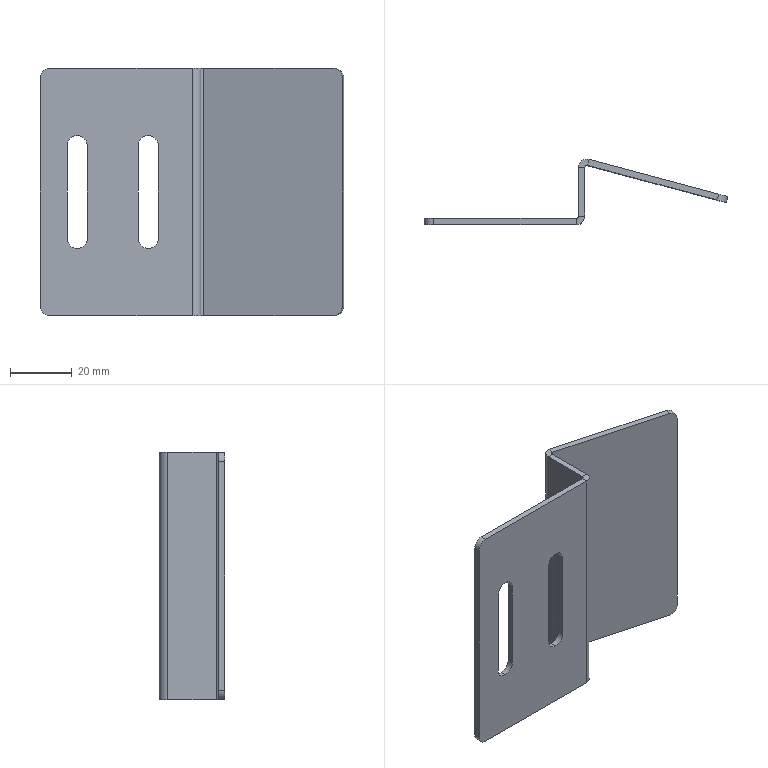Part | STEP file | 1 solid | 36 faces | box 98.296 x 21.17 x 80 mm | volume 17841 mm3 | plane 22 | cylinder 14 | commonest cylinder face diameters 6.5 x6 6 x4 1.473 x2 5.473 x2